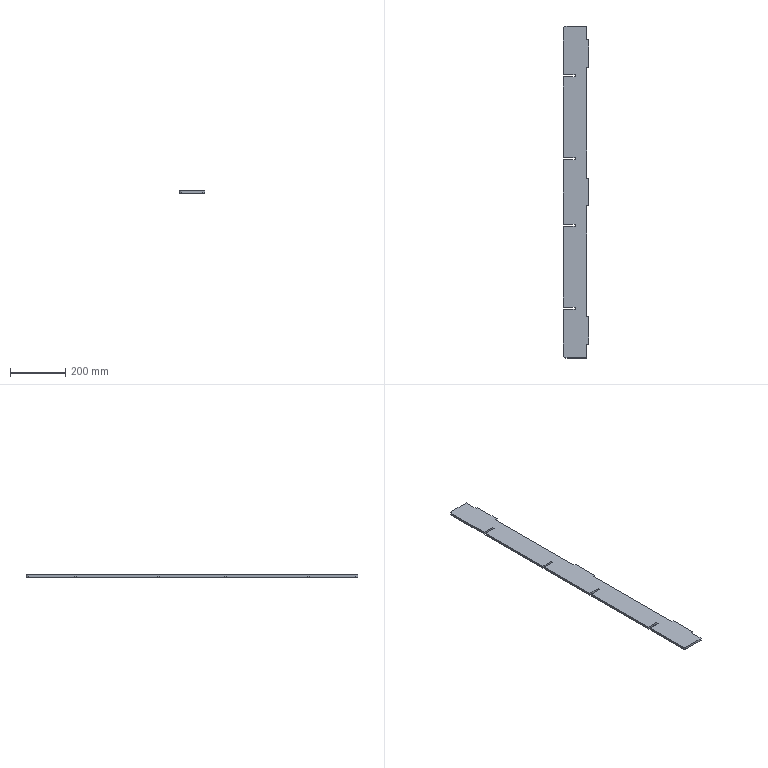Part | SolidWorks | features FlatPattern 1, SMBaseFlange 1, SheetMetal 1 | 1 solid | 36 faces | box 92.5 x 1200 x 8 mm | volume 822649 mm3 | plane 34 | cylinder 2 | commonest cylinder face diameters 20 x2
STEP:
#1=CARTESIAN_POINT('',(982.506,-540.938,0.));
#2=VERTEX_POINT('',#1);
#3=CARTESIAN_POINT('',(982.506,-490.938,0.));
#4=VERTEX_POINT('',#3);
#5=CARTESIAN_POINT('',(982.506,-490.938,0.));
#6=DIRECTION('',(0.,1.,0.));
#7=VECTOR('',#6,1000.);
#8=LINE('',#5,#7);
#9=EDGE_CURVE('',#2,#4,#8,.T.);
#10=ORIENTED_EDGE('',*,*,#9,.F.);
#11=CARTESIAN_POINT('',(982.506,-540.938,-8.));
#12=VERTEX_POINT('',#11);
#13=CARTESIAN_POINT('',(982.506,-540.938,-8.));
#14=DIRECTION('',(0.,0.,1.));
#15=VECTOR('',#14,1000.);
#16=LINE('',#13,#15);
#17=EDGE_CURVE('',#12,#2,#16,.T.);
#18=ORIENTED_EDGE('',*,*,#17,.F.);
#19=CARTESIAN_POINT('',(982.506,-490.938,-8.));
#20=VERTEX_POINT('',#19);
#21=CARTESIAN_POINT('',(982.506,-490.938,-8.));
#22=DIRECTION('',(0.,1.,0.));
#23=VECTOR('',#22,1000.);
#24=LINE('',#21,#23);
#25=EDGE_CURVE('',#12,#20,#24,.T.);
#26=ORIENTED_EDGE('',*,*,#25,.T.);
#27=CARTESIAN_POINT('',(982.506,-490.938,-8.));
#28=DIRECTION('',(0.,0.,1.));
#29=VECTOR('',#28,1000.);
#30=LINE('',#27,#29);
#31=EDGE_CURVE('',#20,#4,#30,.T.);
#32=ORIENTED_EDGE('',*,*,#31,.T.);
#33=EDGE_LOOP('',(#10,#18,#26,#32));
#34=FACE_OUTER_BOUND('',#33,.T.);
#35=CARTESIAN_POINT('',(982.506,-490.938,-8.));
#36=DIRECTION('',(1.,0.,0.));
#37=DIRECTION('',(0.,1.,0.));
#38=AXIS2_PLACEMENT_3D('',#35,#36,#37);
#39=PLANE('',#38);
#40=ADVANCED_FACE('',(#34),#39,.T.);
#41=CARTESIAN_POINT('',(907.506,-540.938,0.));
#42=VERTEX_POINT('',#41);
#43=CARTESIAN_POINT('',(982.506,-540.938,0.));
#44=DIRECTION('',(1.,0.,0.));
#45=VECTOR('',#44,1000.);
#46=LINE('',#43,#45);
#47=EDGE_CURVE('',#42,#2,#46,.T.);
#48=ORIENTED_EDGE('',*,*,#47,.F.);
#49=CARTESIAN_POINT('',(907.506,-540.938,-8.));
#50=VERTEX_POINT('',#49);
#51=CARTESIAN_POINT('',(907.506,-540.938,-8.));
#52=DIRECTION('',(0.,0.,1.));
#53=VECTOR('',#52,1000.);
#54=LINE('',#51,#53);
#55=EDGE_CURVE('',#50,#42,#54,.T.);
#56=ORIENTED_EDGE('',*,*,#55,.F.);
#57=CARTESIAN_POINT('',(982.506,-540.938,-8.));
#58=DIRECTION('',(1.,0.,0.));
#59=VECTOR('',#58,1000.);
#60=LINE('',#57,#59);
#61=EDGE_CURVE('',#50,#12,#60,.T.);
#62=ORIENTED_EDGE('',*,*,#61,.T.);
#63=ORIENTED_EDGE('',*,*,#17,.T.);
#64=EDGE_LOOP('',(#48,#56,#62,#63));
#65=FACE_OUTER_BOUND('',#64,.T.);
#66=CARTESIAN_POINT('',(982.506,-540.938,-8.));
#67=DIRECTION('',(0.,-1.,0.));
#68=DIRECTION('',(0.,0.,-1.));
#69=AXIS2_PLACEMENT_3D('',#66,#67,#68);
#70=PLANE('',#69);
#71=ADVANCED_FACE('',(#65),#70,.T.);
#72=CARTESIAN_POINT('',(897.506,-530.938,0.));
#73=VERTEX_POINT('',#72);
#74=CARTESIAN_POINT('',(907.506,-530.938,0.));
#75=DIRECTION('',(0.,0.,1.));
#76=DIRECTION('',(-1.,0.,0.));
#77=AXIS2_PLACEMENT_3D('',#74,#75,#76);
#78=CIRCLE('',#77,10.);
#79=EDGE_CURVE('',#73,#42,#78,.T.);
#80=ORIENTED_EDGE('',*,*,#79,.F.);
#81=CARTESIAN_POINT('',(897.506,-530.938,-8.));
#82=VERTEX_POINT('',#81);
#83=CARTESIAN_POINT('',(897.506,-530.938,-8.));
#84=DIRECTION('',(0.,0.,1.));
#85=VECTOR('',#84,1000.);
#86=LINE('',#83,#85);
#87=EDGE_CURVE('',#82,#73,#86,.T.);
#88=ORIENTED_EDGE('',*,*,#87,.F.);
#89=CARTESIAN_POINT('',(907.506,-530.938,-8.));
#90=DIRECTION('',(0.,0.,1.));
#91=DIRECTION('',(-1.,0.,0.));
#92=AXIS2_PLACEMENT_3D('',#89,#90,#91);
#93=CIRCLE('',#92,10.);
#94=EDGE_CURVE('',#82,#50,#93,.T.);
#95=ORIENTED_EDGE('',*,*,#94,.T.);
#96=ORIENTED_EDGE('',*,*,#55,.T.);
#97=EDGE_LOOP('',(#80,#88,#95,#96));
#98=FACE_OUTER_BOUND('',#97,.T.);
#99=CARTESIAN_POINT('',(907.506,-530.938,-8.));
#100=DIRECTION('',(0.,0.,1.));
#101=DIRECTION('',(1.,0.,0.));
#102=AXIS2_PLACEMENT_3D('',#99,#100,#101);
#103=CYLINDRICAL_SURFACE('',#102,10.);
#104=ADVANCED_FACE('',(#98),#103,.T.);
#105=CARTESIAN_POINT('',(897.506,-364.938,0.));
#106=VERTEX_POINT('',#105);
#107=CARTESIAN_POINT('',(897.506,-530.938,0.));
#108=DIRECTION('',(0.,-1.,0.));
#109=VECTOR('',#108,1000.);
#110=LINE('',#107,#109);
#111=EDGE_CURVE('',#106,#73,#110,.T.);
#112=ORIENTED_EDGE('',*,*,#111,.F.);
#113=CARTESIAN_POINT('',(897.506,-364.938,-8.));
#114=VERTEX_POINT('',#113);
#115=CARTESIAN_POINT('',(897.506,-364.938,-8.));
#116=DIRECTION('',(0.,0.,1.));
#117=VECTOR('',#116,1000.);
#118=LINE('',#115,#117);
#119=EDGE_CURVE('',#114,#106,#118,.T.);
#120=ORIENTED_EDGE('',*,*,#119,.F.);
#121=CARTESIAN_POINT('',(897.506,-530.938,-8.));
#122=DIRECTION('',(0.,-1.,0.));
#123=VECTOR('',#122,1000.);
#124=LINE('',#121,#123);
#125=EDGE_CURVE('',#114,#82,#124,.T.);
#126=ORIENTED_EDGE('',*,*,#125,.T.);
#127=ORIENTED_EDGE('',*,*,#87,.T.);
#128=EDGE_LOOP('',(#112,#120,#126,#127));
#129=FACE_OUTER_BOUND('',#128,.T.);
#130=CARTESIAN_POINT('',(897.506,-530.938,-8.));
#131=DIRECTION('',(-1.,0.,0.));
#132=DIRECTION('',(0.,0.,1.));
#133=AXIS2_PLACEMENT_3D('',#130,#131,#132);
#134=PLANE('',#133);
#135=ADVANCED_FACE('',(#129),#134,.T.);
#136=CARTESIAN_POINT('',(940.506,-364.938,0.));
#137=VERTEX_POINT('',#136);
#138=CARTESIAN_POINT('',(940.506,-364.938,0.));
#139=DIRECTION('',(-1.,0.,0.));
#140=VECTOR('',#139,1000.);
#141=LINE('',#138,#140);
#142=EDGE_CURVE('',#137,#106,#141,.T.);
#143=ORIENTED_EDGE('',*,*,#142,.F.);
#144=CARTESIAN_POINT('',(940.506,-364.938,-8.));
#145=VERTEX_POINT('',#144);
#146=CARTESIAN_POINT('',(940.506,-364.938,-8.));
#147=DIRECTION('',(0.,0.,1.));
#148=VECTOR('',#147,1000.);
#149=LINE('',#146,#148);
#150=EDGE_CURVE('',#145,#137,#149,.T.);
#151=ORIENTED_EDGE('',*,*,#150,.F.);
#152=CARTESIAN_POINT('',(940.506,-364.938,-8.));
#153=DIRECTION('',(-1.,0.,0.));
#154=VECTOR('',#153,1000.);
#155=LINE('',#152,#154);
#156=EDGE_CURVE('',#145,#114,#155,.T.);
#157=ORIENTED_EDGE('',*,*,#156,.T.);
#158=ORIENTED_EDGE('',*,*,#119,.T.);
#159=EDGE_LOOP('',(#143,#151,#157,#158));
#160=FACE_OUTER_BOUND('',#159,.T.);
#161=CARTESIAN_POINT('',(940.506,-364.938,-8.));
#162=DIRECTION('',(0.,1.,0.));
#163=DIRECTION('',(0.,0.,1.));
#164=AXIS2_PLACEMENT_3D('',#161,#162,#163);
#165=PLANE('',#164);
#166=ADVANCED_FACE('',(#160),#165,.T.);
#167=CARTESIAN_POINT('',(940.506,-356.938,0.));
#168=VERTEX_POINT('',#167);
#169=CARTESIAN_POINT('',(940.506,-356.938,0.));
#170=DIRECTION('',(0.,-1.,0.));
#171=VECTOR('',#170,1000.);
#172=LINE('',#169,#171);
#173=EDGE_CURVE('',#168,#137,#172,.T.);
#174=ORIENTED_EDGE('',*,*,#173,.F.);
#175=CARTESIAN_POINT('',(940.506,-356.938,-8.));
#176=VERTEX_POINT('',#175);
#177=CARTESIAN_POINT('',(940.506,-356.938,-8.));
#178=DIRECTION('',(0.,0.,1.));
#179=VECTOR('',#178,1000.);
#180=LINE('',#177,#179);
#181=EDGE_CURVE('',#176,#168,#180,.T.);
#182=ORIENTED_EDGE('',*,*,#181,.F.);
#183=CARTESIAN_POINT('',(940.506,-356.938,-8.));
#184=DIRECTION('',(0.,-1.,0.));
#185=VECTOR('',#184,1000.);
#186=LINE('',#183,#185);
#187=EDGE_CURVE('',#176,#145,#186,.T.);
#188=ORIENTED_EDGE('',*,*,#187,.T.);
#189=ORIENTED_EDGE('',*,*,#150,.T.);
#190=EDGE_LOOP('',(#174,#182,#188,#189));
#191=FACE_OUTER_BOUND('',#190,.T.);
#192=CARTESIAN_POINT('',(940.506,-356.938,-8.));
#193=DIRECTION('',(-1.,0.,0.));
#194=DIRECTION('',(0.,0.,1.));
#195=AXIS2_PLACEMENT_3D('',#192,#193,#194);
#196=PLANE('',#195);
#197=ADVANCED_FACE('',(#191),#196,.T.);
#198=CARTESIAN_POINT('',(897.506,-356.938,0.));
#199=VERTEX_POINT('',#198);
#200=CARTESIAN_POINT('',(897.506,-356.938,0.));
#201=DIRECTION('',(1.,0.,0.));
#202=VECTOR('',#201,1000.);
#203=LINE('',#200,#202);
#204=EDGE_CURVE('',#199,#168,#203,.T.);
#205=ORIENTED_EDGE('',*,*,#204,.F.);
#206=CARTESIAN_POINT('',(897.506,-356.938,-8.));
#207=VERTEX_POINT('',#206);
#208=CARTESIAN_POINT('',(897.506,-356.938,-8.));
#209=DIRECTION('',(0.,0.,1.));
#210=VECTOR('',#209,1000.);
#211=LINE('',#208,#210);
#212=EDGE_CURVE('',#207,#199,#211,.T.);
#213=ORIENTED_EDGE('',*,*,#212,.F.);
#214=CARTESIAN_POINT('',(897.506,-356.938,-8.));
#215=DIRECTION('',(1.,0.,0.));
#216=VECTOR('',#215,1000.);
#217=LINE('',#214,#216);
#218=EDGE_CURVE('',#207,#176,#217,.T.);
#219=ORIENTED_EDGE('',*,*,#218,.T.);
#220=ORIENTED_EDGE('',*,*,#181,.T.);
#221=EDGE_LOOP('',(#205,#213,#219,#220));
#222=FACE_OUTER_BOUND('',#221,.T.);
#223=CARTESIAN_POINT('',(897.506,-356.938,-8.));
#224=DIRECTION('',(0.,-1.,0.));
#225=DIRECTION('',(0.,0.,-1.));
#226=AXIS2_PLACEMENT_3D('',#223,#224,#225);
#227=PLANE('',#226);
#228=ADVANCED_FACE('',(#222),#227,.T.);
#229=CARTESIAN_POINT('',(897.506,-64.938,0.));
#230=VERTEX_POINT('',#229);
#231=CARTESIAN_POINT('',(897.506,-356.938,0.));
#232=DIRECTION('',(0.,-1.,0.));
#233=VECTOR('',#232,1000.);
#234=LINE('',#231,#233);
#235=EDGE_CURVE('',#230,#199,#234,.T.);
#236=ORIENTED_EDGE('',*,*,#235,.F.);
#237=CARTESIAN_POINT('',(897.506,-64.938,-8.));
#238=VERTEX_POINT('',#237);
#239=CARTESIAN_POINT('',(897.506,-64.938,-8.));
#240=DIRECTION('',(0.,0.,1.));
#241=VECTOR('',#240,1000.);
#242=LINE('',#239,#241);
#243=EDGE_CURVE('',#238,#230,#242,.T.);
#244=ORIENTED_EDGE('',*,*,#243,.F.);
#245=CARTESIAN_POINT('',(897.506,-356.938,-8.));
#246=DIRECTION('',(0.,-1.,0.));
#247=VECTOR('',#246,1000.);
#248=LINE('',#245,#247);
#249=EDGE_CURVE('',#238,#207,#248,.T.);
#250=ORIENTED_EDGE('',*,*,#249,.T.);
#251=ORIENTED_EDGE('',*,*,#212,.T.);
#252=EDGE_LOOP('',(#236,#244,#250,#251));
#253=FACE_OUTER_BOUND('',#252,.T.);
#254=CARTESIAN_POINT('',(897.506,-356.938,-8.));
#255=DIRECTION('',(-1.,0.,0.));
#256=DIRECTION('',(0.,0.,1.));
#257=AXIS2_PLACEMENT_3D('',#254,#255,#256);
#258=PLANE('',#257);
#259=ADVANCED_FACE('',(#253),#258,.T.);
#260=CARTESIAN_POINT('',(940.506,-64.938,0.));
#261=VERTEX_POINT('',#260);
#262=CARTESIAN_POINT('',(940.506,-64.938,0.));
#263=DIRECTION('',(-1.,0.,0.));
#264=VECTOR('',#263,1000.);
#265=LINE('',#262,#264);
#266=EDGE_CURVE('',#261,#230,#265,.T.);
#267=ORIENTED_EDGE('',*,*,#266,.F.);
#268=CARTESIAN_POINT('',(940.506,-64.938,-8.));
#269=VERTEX_POINT('',#268);
#270=CARTESIAN_POINT('',(940.506,-64.938,-8.));
#271=DIRECTION('',(0.,0.,1.));
#272=VECTOR('',#271,1000.);
#273=LINE('',#270,#272);
#274=EDGE_CURVE('',#269,#261,#273,.T.);
#275=ORIENTED_EDGE('',*,*,#274,.F.);
#276=CARTESIAN_POINT('',(940.506,-64.938,-8.));
#277=DIRECTION('',(-1.,0.,0.));
#278=VECTOR('',#277,1000.);
#279=LINE('',#276,#278);
#280=EDGE_CURVE('',#269,#238,#279,.T.);
#281=ORIENTED_EDGE('',*,*,#280,.T.);
#282=ORIENTED_EDGE('',*,*,#243,.T.);
#283=EDGE_LOOP('',(#267,#275,#281,#282));
#284=FACE_OUTER_BOUND('',#283,.T.);
#285=CARTESIAN_POINT('',(940.506,-64.938,-8.));
#286=DIRECTION('',(0.,1.,0.));
#287=DIRECTION('',(0.,0.,1.));
#288=AXIS2_PLACEMENT_3D('',#285,#286,#287);
#289=PLANE('',#288);
#290=ADVANCED_FACE('',(#284),#289,.T.);
#291=CARTESIAN_POINT('',(940.506,-56.938,0.));
#292=VERTEX_POINT('',#291);
#293=CARTESIAN_POINT('',(940.506,-56.938,0.));
#294=DIRECTION('',(0.,-1.,0.));
#295=VECTOR('',#294,1000.);
#296=LINE('',#293,#295);
#297=EDGE_CURVE('',#292,#261,#296,.T.);
#298=ORIENTED_EDGE('',*,*,#297,.F.);
#299=CARTESIAN_POINT('',(940.506,-56.938,-8.));
#300=VERTEX_POINT('',#299);
#301=CARTESIAN_POINT('',(940.506,-56.938,-8.));
#302=DIRECTION('',(0.,0.,1.));
#303=VECTOR('',#302,1000.);
#304=LINE('',#301,#303);
#305=EDGE_CURVE('',#300,#292,#304,.T.);
#306=ORIENTED_EDGE('',*,*,#305,.F.);
#307=CARTESIAN_POINT('',(940.506,-56.938,-8.));
#308=DIRECTION('',(0.,-1.,0.));
#309=VECTOR('',#308,1000.);
#310=LINE('',#307,#309);
#311=EDGE_CURVE('',#300,#269,#310,.T.);
#312=ORIENTED_EDGE('',*,*,#311,.T.);
#313=ORIENTED_EDGE('',*,*,#274,.T.);
#314=EDGE_LOOP('',(#298,#306,#312,#313));
#315=FACE_OUTER_BOUND('',#314,.T.);
#316=CARTESIAN_POINT('',(940.506,-56.938,-8.));
#317=DIRECTION('',(-1.,0.,0.));
#318=DIRECTION('',(0.,0.,1.));
#319=AXIS2_PLACEMENT_3D('',#316,#317,#318);
#320=PLANE('',#319);
#321=ADVANCED_FACE('',(#315),#320,.T.);
#322=CARTESIAN_POINT('',(897.506,-56.938,0.));
#323=VERTEX_POINT('',#322);
#324=CARTESIAN_POINT('',(897.506,-56.938,0.));
#325=DIRECTION('',(1.,0.,0.));
#326=VECTOR('',#325,1000.);
#327=LINE('',#324,#326);
#328=EDGE_CURVE('',#323,#292,#327,.T.);
#329=ORIENTED_EDGE('',*,*,#328,.F.);
#330=CARTESIAN_POINT('',(897.506,-56.938,-8.));
#331=VERTEX_POINT('',#330);
#332=CARTESIAN_POINT('',(897.506,-56.938,-8.));
#333=DIRECTION('',(0.,0.,1.));
#334=VECTOR('',#333,1000.);
#335=LINE('',#332,#334);
#336=EDGE_CURVE('',#331,#323,#335,.T.);
#337=ORIENTED_EDGE('',*,*,#336,.F.);
#338=CARTESIAN_POINT('',(897.506,-56.938,-8.));
#339=DIRECTION('',(1.,0.,0.));
#340=VECTOR('',#339,1000.);
#341=LINE('',#338,#340);
#342=EDGE_CURVE('',#331,#300,#341,.T.);
#343=ORIENTED_EDGE('',*,*,#342,.T.);
#344=ORIENTED_EDGE('',*,*,#305,.T.);
#345=EDGE_LOOP('',(#329,#337,#343,#344));
#346=FACE_OUTER_BOUND('',#345,.T.);
#347=CARTESIAN_POINT('',(897.506,-56.938,-8.));
#348=DIRECTION('',(0.,-1.,0.));
#349=DIRECTION('',(0.,0.,-1.));
#350=AXIS2_PLACEMENT_3D('',#347,#348,#349);
#351=PLANE('',#350);
#352=ADVANCED_FACE('',(#346),#351,.T.);
#353=CARTESIAN_POINT('',(897.506,175.062,0.));
#354=VERTEX_POINT('',#353);
#355=CARTESIAN_POINT('',(897.506,-56.938,0.));
#356=DIRECTION('',(0.,-1.,0.));
#357=VECTOR('',#356,1000.);
#358=LINE('',#355,#357);
#359=EDGE_CURVE('',#354,#323,#358,.T.);
#360=ORIENTED_EDGE('',*,*,#359,.F.);
#361=CARTESIAN_POINT('',(897.506,175.062,-8.));
#362=VERTEX_POINT('',#361);
#363=CARTESIAN_POINT('',(897.506,175.062,-8.));
#364=DIRECTION('',(0.,0.,1.));
#365=VECTOR('',#364,1000.);
#366=LINE('',#363,#365);
#367=EDGE_CURVE('',#362,#354,#366,.T.);
#368=ORIENTED_EDGE('',*,*,#367,.F.);
#369=CARTESIAN_POINT('',(897.506,-56.938,-8.));
#370=DIRECTION('',(0.,-1.,0.));
#371=VECTOR('',#370,1000.);
#372=LINE('',#369,#371);
#373=EDGE_CURVE('',#362,#331,#372,.T.);
#374=ORIENTED_EDGE('',*,*,#373,.T.);
#375=ORIENTED_EDGE('',*,*,#336,.T.);
#376=EDGE_LOOP('',(#360,#368,#374,#375));
#377=FACE_OUTER_BOUND('',#376,.T.);
#378=CARTESIAN_POINT('',(897.506,-56.938,-8.));
#379=DIRECTION('',(-1.,0.,0.));
#380=DIRECTION('',(0.,0.,1.));
#381=AXIS2_PLACEMENT_3D('',#378,#379,#380);
#382=PLANE('',#381);
#383=ADVANCED_FACE('',(#377),#382,.T.);
#384=CARTESIAN_POINT('',(940.506,175.062,0.));
#385=VERTEX_POINT('',#384);
#386=CARTESIAN_POINT('',(940.506,175.062,0.));
#387=DIRECTION('',(-1.,0.,0.));
#388=VECTOR('',#387,1000.);
#389=LINE('',#386,#388);
#390=EDGE_CURVE('',#385,#354,#389,.T.);
#391=ORIENTED_EDGE('',*,*,#390,.F.);
#392=CARTESIAN_POINT('',(940.506,175.062,-8.));
#393=VERTEX_POINT('',#392);
#394=CARTESIAN_POINT('',(940.506,175.062,-8.));
#395=DIRECTION('',(0.,0.,1.));
#396=VECTOR('',#395,1000.);
#397=LINE('',#394,#396);
#398=EDGE_CURVE('',#393,#385,#397,.T.);
#399=ORIENTED_EDGE('',*,*,#398,.F.);
#400=CARTESIAN_POINT('',(940.506,175.062,-8.));
#401=DIRECTION('',(-1.,0.,0.));
#402=VECTOR('',#401,1000.);
#403=LINE('',#400,#402);
#404=EDGE_CURVE('',#393,#362,#403,.T.);
#405=ORIENTED_EDGE('',*,*,#404,.T.);
#406=ORIENTED_EDGE('',*,*,#367,.T.);
#407=EDGE_LOOP('',(#391,#399,#405,#406));
#408=FACE_OUTER_BOUND('',#407,.T.);
#409=CARTESIAN_POINT('',(940.506,175.062,-8.));
#410=DIRECTION('',(0.,1.,0.));
#411=DIRECTION('',(0.,0.,1.));
#412=AXIS2_PLACEMENT_3D('',#409,#410,#411);
#413=PLANE('',#412);
#414=ADVANCED_FACE('',(#408),#413,.T.);
#415=CARTESIAN_POINT('',(940.506,183.062,0.));
#416=VERTEX_POINT('',#415);
#417=CARTESIAN_POINT('',(940.506,183.062,0.));
#418=DIRECTION('',(0.,-1.,0.));
#419=VECTOR('',#418,1000.);
#420=LINE('',#417,#419);
#421=EDGE_CURVE('',#416,#385,#420,.T.);
#422=ORIENTED_EDGE('',*,*,#421,.F.);
#423=CARTESIAN_POINT('',(940.506,183.062,-8.));
#424=VERTEX_POINT('',#423);
#425=CARTESIAN_POINT('',(940.506,183.062,-8.));
#426=DIRECTION('',(0.,0.,1.));
#427=VECTOR('',#426,1000.);
#428=LINE('',#425,#427);
#429=EDGE_CURVE('',#424,#416,#428,.T.);
#430=ORIENTED_EDGE('',*,*,#429,.F.);
#431=CARTESIAN_POINT('',(940.506,183.062,-8.));
#432=DIRECTION('',(0.,-1.,0.));
#433=VECTOR('',#432,1000.);
#434=LINE('',#431,#433);
#435=EDGE_CURVE('',#424,#393,#434,.T.);
#436=ORIENTED_EDGE('',*,*,#435,.T.);
#437=ORIENTED_EDGE('',*,*,#398,.T.);
#438=EDGE_LOOP('',(#422,#430,#436,#437));
#439=FACE_OUTER_BOUND('',#438,.T.);
#440=CARTESIAN_POINT('',(940.506,183.062,-8.));
#441=DIRECTION('',(-1.,0.,0.));
#442=DIRECTION('',(0.,0.,1.));
#443=AXIS2_PLACEMENT_3D('',#440,#441,#442);
#444=PLANE('',#443);
#445=ADVANCED_FACE('',(#439),#444,.T.);
#446=CARTESIAN_POINT('',(897.506,183.062,0.));
#447=VERTEX_POINT('',#446);
#448=CARTESIAN_POINT('',(897.506,183.062,0.));
#449=DIRECTION('',(1.,0.,0.));
#450=VECTOR('',#449,1000.);
#451=LINE('',#448,#450);
#452=EDGE_CURVE('',#447,#416,#451,.T.);
#453=ORIENTED_EDGE('',*,*,#452,.F.);
#454=CARTESIAN_POINT('',(897.506,183.062,-8.));
#455=VERTEX_POINT('',#454);
#456=CARTESIAN_POINT('',(897.506,183.062,-8.));
#457=DIRECTION('',(0.,0.,1.));
#458=VECTOR('',#457,1000.);
#459=LINE('',#456,#458);
#460=EDGE_CURVE('',#455,#447,#459,.T.);
#461=ORIENTED_EDGE('',*,*,#460,.F.);
#462=CARTESIAN_POINT('',(897.506,183.062,-8.));
#463=DIRECTION('',(1.,0.,0.));
#464=VECTOR('',#463,1000.);
#465=LINE('',#462,#464);
#466=EDGE_CURVE('',#455,#424,#465,.T.);
#467=ORIENTED_EDGE('',*,*,#466,.T.);
#468=ORIENTED_EDGE('',*,*,#429,.T.);
#469=EDGE_LOOP('',(#453,#461,#467,#468));
#470=FACE_OUTER_BOUND('',#469,.T.);
#471=CARTESIAN_POINT('',(897.506,183.062,-8.));
#472=DIRECTION('',(0.,-1.,0.));
#473=DIRECTION('',(1.,0.,0.));
#474=AXIS2_PLACEMENT_3D('',#471,#472,#473);
#475=PLANE('',#474);
#476=ADVANCED_FACE('',(#470),#475,.T.);
#477=CARTESIAN_POINT('',(897.506,475.062,0.));
#478=VERTEX_POINT('',#477);
#479=CARTESIAN_POINT('',(897.506,183.062,0.));
#480=DIRECTION('',(0.,-1.,0.));
#481=VECTOR('',#480,1000.);
#482=LINE('',#479,#481);
#483=EDGE_CURVE('',#478,#447,#482,.T.);
#484=ORIENTED_EDGE('',*,*,#483,.F.);
#485=CARTESIAN_POINT('',(897.506,475.062,-8.));
#486=VERTEX_POINT('',#485);
#487=CARTESIAN_POINT('',(897.506,475.062,-8.));
#488=DIRECTION('',(0.,0.,1.));
#489=VECTOR('',#488,1000.);
#490=LINE('',#487,#489);
#491=EDGE_CURVE('',#486,#478,#490,.T.);
#492=ORIENTED_EDGE('',*,*,#491,.F.);
#493=CARTESIAN_POINT('',(897.506,183.062,-8.));
#494=DIRECTION('',(0.,-1.,0.));
#495=VECTOR('',#494,1000.);
#496=LINE('',#493,#495);
#497=EDGE_CURVE('',#486,#455,#496,.T.);
#498=ORIENTED_EDGE('',*,*,#497,.T.);
#499=ORIENTED_EDGE('',*,*,#460,.T.);
#500=EDGE_LOOP('',(#484,#492,#498,#499));
#501=FACE_OUTER_BOUND('',#500,.T.);
#502=CARTESIAN_POINT('',(897.506,183.062,-8.));
#503=DIRECTION('',(-1.,0.,0.));
#504=DIRECTION('',(0.,0.,1.));
#505=AXIS2_PLACEMENT_3D('',#502,#503,#504);
#506=PLANE('',#505);
#507=ADVANCED_FACE('',(#501),#506,.T.);
#508=CARTESIAN_POINT('',(940.506,475.062,0.));
#509=VERTEX_POINT('',#508);
#510=CARTESIAN_POINT('',(940.506,475.062,0.));
#511=DIRECTION('',(-1.,0.,0.));
#512=VECTOR('',#511,1000.);
#513=LINE('',#510,#512);
#514=EDGE_CURVE('',#509,#478,#513,.T.);
#515=ORIENTED_EDGE('',*,*,#514,.F.);
#516=CARTESIAN_POINT('',(940.506,475.062,-8.));
#517=VERTEX_POINT('',#516);
#518=CARTESIAN_POINT('',(940.506,475.062,-8.));
#519=DIRECTION('',(0.,0.,1.));
#520=VECTOR('',#519,1000.);
#521=LINE('',#518,#520);
#522=EDGE_CURVE('',#517,#509,#521,.T.);
#523=ORIENTED_EDGE('',*,*,#522,.F.);
#524=CARTESIAN_POINT('',(940.506,475.062,-8.));
#525=DIRECTION('',(-1.,0.,0.));
#526=VECTOR('',#525,1000.);
#527=LINE('',#524,#526);
#528=EDGE_CURVE('',#517,#486,#527,.T.);
#529=ORIENTED_EDGE('',*,*,#528,.T.);
#530=ORIENTED_EDGE('',*,*,#491,.T.);
#531=EDGE_LOOP('',(#515,#523,#529,#530));
#532=FACE_OUTER_BOUND('',#531,.T.);
#533=CARTESIAN_POINT('',(940.506,475.062,-8.));
#534=DIRECTION('',(0.,1.,0.));
#535=DIRECTION('',(-1.,0.,0.));
#536=AXIS2_PLACEMENT_3D('',#533,#534,#535);
#537=PLANE('',#536);
#538=ADVANCED_FACE('',(#532),#537,.T.);
#539=CARTESIAN_POINT('',(940.506,483.062,0.));
#540=VERTEX_POINT('',#539);
#541=CARTESIAN_POINT('',(940.506,483.062,0.));
#542=DIRECTION('',(0.,-1.,0.));
#543=VECTOR('',#542,1000.);
#544=LINE('',#541,#543);
#545=EDGE_CURVE('',#540,#509,#544,.T.);
#546=ORIENTED_EDGE('',*,*,#545,.F.);
#547=CARTESIAN_POINT('',(940.506,483.062,-8.));
#548=VERTEX_POINT('',#547);
#549=CARTESIAN_POINT('',(940.506,483.062,-8.));
#550=DIRECTION('',(0.,0.,1.));
#551=VECTOR('',#550,1000.);
#552=LINE('',#549,#551);
#553=EDGE_CURVE('',#548,#540,#552,.T.);
#554=ORIENTED_EDGE('',*,*,#553,.F.);
#555=CARTESIAN_POINT('',(940.506,483.062,-8.));
#556=DIRECTION('',(0.,-1.,0.));
#557=VECTOR('',#556,1000.);
#558=LINE('',#555,#557);
#559=EDGE_CURVE('',#548,#517,#558,.T.);
#560=ORIENTED_EDGE('',*,*,#559,.T.);
#561=ORIENTED_EDGE('',*,*,#522,.T.);
#562=EDGE_LOOP('',(#546,#554,#560,#561));
#563=FACE_OUTER_BOUND('',#562,.T.);
#564=CARTESIAN_POINT('',(940.506,483.062,-8.));
#565=DIRECTION('',(-1.,0.,0.));
#566=DIRECTION('',(0.,0.,1.));
#567=AXIS2_PLACEMENT_3D('',#564,#565,#566);
#568=PLANE('',#567);
#569=ADVANCED_FACE('',(#563),#568,.T.);
#570=CARTESIAN_POINT('',(897.506,483.062,0.));
#571=VERTEX_POINT('',#570);
#572=CARTESIAN_POINT('',(897.506,483.062,0.));
#573=DIRECTION('',(1.,0.,0.));
#574=VECTOR('',#573,1000.);
#575=LINE('',#572,#574);
#576=EDGE_CURVE('',#571,#540,#575,.T.);
#577=ORIENTED_EDGE('',*,*,#576,.F.);
#578=CARTESIAN_POINT('',(897.506,483.062,-8.));
#579=VERTEX_POINT('',#578);
#580=CARTESIAN_POINT('',(897.506,483.062,-8.));
#581=DIRECTION('',(0.,0.,1.));
#582=VECTOR('',#581,1000.);
#583=LINE('',#580,#582);
#584=EDGE_CURVE('',#579,#571,#583,.T.);
#585=ORIENTED_EDGE('',*,*,#584,.F.);
#586=CARTESIAN_POINT('',(897.506,483.062,-8.));
#587=DIRECTION('',(1.,0.,0.));
#588=VECTOR('',#587,1000.);
#589=LINE('',#586,#588);
#590=EDGE_CURVE('',#579,#548,#589,.T.);
#591=ORIENTED_EDGE('',*,*,#590,.T.);
#592=ORIENTED_EDGE('',*,*,#553,.T.);
#593=EDGE_LOOP('',(#577,#585,#591,#592));
#594=FACE_OUTER_BOUND('',#593,.T.);
#595=CARTESIAN_POINT('',(897.506,483.062,-8.));
#596=DIRECTION('',(0.,-1.,0.));
#597=DIRECTION('',(1.,0.,0.));
#598=AXIS2_PLACEMENT_3D('',#595,#596,#597);
#599=PLANE('',#598);
#600=ADVANCED_FACE('',(#594),#599,.T.);
#601=CARTESIAN_POINT('',(897.506,649.062,0.));
#602=VERTEX_POINT('',#601);
#603=CARTESIAN_POINT('',(897.506,483.062,0.));
#604=DIRECTION('',(0.,-1.,0.));
#605=VECTOR('',#604,1000.);
#606=LINE('',#603,#605);
#607=EDGE_CURVE('',#602,#571,#606,.T.);
#608=ORIENTED_EDGE('',*,*,#607,.F.);
#609=CARTESIAN_POINT('',(897.506,649.062,-8.));
#610=VERTEX_POINT('',#609);
#611=CARTESIAN_POINT('',(897.506,649.062,-8.));
#612=DIRECTION('',(0.,0.,1.));
#613=VECTOR('',#612,1000.);
#614=LINE('',#611,#613);
#615=EDGE_CURVE('',#610,#602,#614,.T.);
#616=ORIENTED_EDGE('',*,*,#615,.F.);
#617=CARTESIAN_POINT('',(897.506,483.062,-8.));
#618=DIRECTION('',(0.,-1.,0.));
#619=VECTOR('',#618,1000.);
#620=LINE('',#617,#619);
#621=EDGE_CURVE('',#610,#579,#620,.T.);
#622=ORIENTED_EDGE('',*,*,#621,.T.);
#623=ORIENTED_EDGE('',*,*,#584,.T.);
#624=EDGE_LOOP('',(#608,#616,#622,#623));
#625=FACE_OUTER_BOUND('',#624,.T.);
#626=CARTESIAN_POINT('',(897.506,483.062,-8.));
#627=DIRECTION('',(-1.,0.,0.));
#628=DIRECTION('',(0.,0.,1.));
#629=AXIS2_PLACEMENT_3D('',#626,#627,#628);
#630=PLANE('',#629);
#631=ADVANCED_FACE('',(#625),#630,.T.);
#632=CARTESIAN_POINT('',(907.506,659.062,0.));
#633=VERTEX_POINT('',#632);
#634=CARTESIAN_POINT('',(907.506,649.062,0.));
#635=DIRECTION('',(0.,0.,1.));
#636=DIRECTION('',(-1.,0.,0.));
#637=AXIS2_PLACEMENT_3D('',#634,#635,#636);
#638=CIRCLE('',#637,10.);
#639=EDGE_CURVE('',#633,#602,#638,.T.);
#640=ORIENTED_EDGE('',*,*,#639,.F.);
#641=CARTESIAN_POINT('',(907.506,659.062,-8.));
#642=VERTEX_POINT('',#641);
#643=CARTESIAN_POINT('',(907.506,659.062,-8.));
#644=DIRECTION('',(0.,0.,1.));
#645=VECTOR('',#644,1000.);
#646=LINE('',#643,#645);
#647=EDGE_CURVE('',#642,#633,#646,.T.);
#648=ORIENTED_EDGE('',*,*,#647,.F.);
#649=CARTESIAN_POINT('',(907.506,649.062,-8.));
#650=DIRECTION('',(0.,0.,1.));
#651=DIRECTION('',(-1.,0.,0.));
#652=AXIS2_PLACEMENT_3D('',#649,#650,#651);
#653=CIRCLE('',#652,10.);
#654=EDGE_CURVE('',#642,#610,#653,.T.);
#655=ORIENTED_EDGE('',*,*,#654,.T.);
#656=ORIENTED_EDGE('',*,*,#615,.T.);
#657=EDGE_LOOP('',(#640,#648,#655,#656));
#658=FACE_OUTER_BOUND('',#657,.T.);
#659=CARTESIAN_POINT('',(907.506,649.062,-8.));
#660=DIRECTION('',(0.,0.,1.));
#661=DIRECTION('',(1.,0.,0.));
#662=AXIS2_PLACEMENT_3D('',#659,#660,#661);
#663=CYLINDRICAL_SURFACE('',#662,10.);
#664=ADVANCED_FACE('',(#658),#663,.T.);
#665=CARTESIAN_POINT('',(982.506,659.062,0.));
#666=VERTEX_POINT('',#665);
#667=CARTESIAN_POINT('',(907.506,659.062,0.));
#668=DIRECTION('',(-1.,0.,0.));
#669=VECTOR('',#668,1000.);
#670=LINE('',#667,#669);
#671=EDGE_CURVE('',#666,#633,#670,.T.);
#672=ORIENTED_EDGE('',*,*,#671,.F.);
#673=CARTESIAN_POINT('',(982.506,659.062,-8.));
#674=VERTEX_POINT('',#673);
#675=CARTESIAN_POINT('',(982.506,659.062,-8.));
#676=DIRECTION('',(0.,0.,1.));
#677=VECTOR('',#676,1000.);
#678=LINE('',#675,#677);
#679=EDGE_CURVE('',#674,#666,#678,.T.);
#680=ORIENTED_EDGE('',*,*,#679,.F.);
#681=CARTESIAN_POINT('',(907.506,659.062,-8.));
#682=DIRECTION('',(-1.,0.,0.));
#683=VECTOR('',#682,1000.);
#684=LINE('',#681,#683);
#685=EDGE_CURVE('',#674,#642,#684,.T.);
#686=ORIENTED_EDGE('',*,*,#685,.T.);
#687=ORIENTED_EDGE('',*,*,#647,.T.);
#688=EDGE_LOOP('',(#672,#680,#686,#687));
#689=FACE_OUTER_BOUND('',#688,.T.);
#690=CARTESIAN_POINT('',(907.506,659.062,-8.));
#691=DIRECTION('',(0.,1.,0.));
#692=DIRECTION('',(0.,0.,1.));
#693=AXIS2_PLACEMENT_3D('',#690,#691,#692);
#694=PLANE('',#693);
#695=ADVANCED_FACE('',(#689),#694,.T.);
#696=CARTESIAN_POINT('',(982.506,609.062,0.));
#697=VERTEX_POINT('',#696);
#698=CARTESIAN_POINT('',(982.506,659.062,0.));
#699=DIRECTION('',(0.,1.,0.));
#700=VECTOR('',#699,1000.);
#701=LINE('',#698,#700);
#702=EDGE_CURVE('',#697,#666,#701,.T.);
#703=ORIENTED_EDGE('',*,*,#702,.F.);
#704=CARTESIAN_POINT('',(982.506,609.062,-8.));
#705=VERTEX_POINT('',#704);
#706=CARTESIAN_POINT('',(982.506,609.062,-8.));
#707=DIRECTION('',(0.,0.,1.));
#708=VECTOR('',#707,1000.);
#709=LINE('',#706,#708);
#710=EDGE_CURVE('',#705,#697,#709,.T.);
#711=ORIENTED_EDGE('',*,*,#710,.F.);
#712=CARTESIAN_POINT('',(982.506,659.062,-8.));
#713=DIRECTION('',(0.,1.,0.));
#714=VECTOR('',#713,1000.);
#715=LINE('',#712,#714);
#716=EDGE_CURVE('',#705,#674,#715,.T.);
#717=ORIENTED_EDGE('',*,*,#716,.T.);
#718=ORIENTED_EDGE('',*,*,#679,.T.);
#719=EDGE_LOOP('',(#703,#711,#717,#718));
#720=FACE_OUTER_BOUND('',#719,.T.);
#721=CARTESIAN_POINT('',(982.506,659.062,-8.));
#722=DIRECTION('',(1.,0.,0.));
#723=DIRECTION('',(0.,1.,0.));
#724=AXIS2_PLACEMENT_3D('',#721,#722,#723);
#725=PLANE('',#724);
#726=ADVANCED_FACE('',(#720),#725,.T.);
#727=CARTESIAN_POINT('',(990.006,609.062,0.));
#728=VERTEX_POINT('',#727);
#729=CARTESIAN_POINT('',(982.506,609.062,0.));
#730=DIRECTION('',(-1.,0.,0.));
#731=VECTOR('',#730,1000.);
#732=LINE('',#729,#731);
#733=EDGE_CURVE('',#728,#697,#732,.T.);
#734=ORIENTED_EDGE('',*,*,#733,.F.);
#735=CARTESIAN_POINT('',(990.006,609.062,-8.));
#736=VERTEX_POINT('',#735);
#737=CARTESIAN_POINT('',(990.006,609.062,-8.));
#738=DIRECTION('',(0.,0.,1.));
#739=VECTOR('',#738,1000.);
#740=LINE('',#737,#739);
#741=EDGE_CURVE('',#736,#728,#740,.T.);
#742=ORIENTED_EDGE('',*,*,#741,.F.);
#743=CARTESIAN_POINT('',(982.506,609.062,-8.));
#744=DIRECTION('',(-1.,0.,0.));
#745=VECTOR('',#744,1000.);
#746=LINE('',#743,#745);
#747=EDGE_CURVE('',#736,#705,#746,.T.);
#748=ORIENTED_EDGE('',*,*,#747,.T.);
#749=ORIENTED_EDGE('',*,*,#710,.T.);
#750=EDGE_LOOP('',(#734,#742,#748,#749));
#751=FACE_OUTER_BOUND('',#750,.T.);
#752=CARTESIAN_POINT('',(982.506,609.062,-8.));
#753=DIRECTION('',(0.,1.,0.));
#754=DIRECTION('',(0.,0.,1.));
#755=AXIS2_PLACEMENT_3D('',#752,#753,#754);
#756=PLANE('',#755);
#757=ADVANCED_FACE('',(#751),#756,.T.);
#758=CARTESIAN_POINT('',(990.006,509.062,0.));
#759=VERTEX_POINT('',#758);
#760=CARTESIAN_POINT('',(990.006,609.062,0.));
#761=DIRECTION('',(0.,1.,0.));
#762=VECTOR('',#761,1000.);
#763=LINE('',#760,#762);
#764=EDGE_CURVE('',#759,#728,#763,.T.);
#765=ORIENTED_EDGE('',*,*,#764,.F.);
#766=CARTESIAN_POINT('',(990.006,509.062,-8.));
#767=VERTEX_POINT('',#766);
#768=CARTESIAN_POINT('',(990.006,509.062,-8.));
#769=DIRECTION('',(0.,0.,1.));
#770=VECTOR('',#769,1000.);
#771=LINE('',#768,#770);
#772=EDGE_CURVE('',#767,#759,#771,.T.);
#773=ORIENTED_EDGE('',*,*,#772,.F.);
#774=CARTESIAN_POINT('',(990.006,609.062,-8.));
#775=DIRECTION('',(0.,1.,0.));
#776=VECTOR('',#775,1000.);
#777=LINE('',#774,#776);
#778=EDGE_CURVE('',#767,#736,#777,.T.);
#779=ORIENTED_EDGE('',*,*,#778,.T.);
#780=ORIENTED_EDGE('',*,*,#741,.T.);
#781=EDGE_LOOP('',(#765,#773,#779,#780));
#782=FACE_OUTER_BOUND('',#781,.T.);
#783=CARTESIAN_POINT('',(990.006,609.062,-8.));
#784=DIRECTION('',(1.,0.,0.));
#785=DIRECTION('',(0.,0.,-1.));
#786=AXIS2_PLACEMENT_3D('',#783,#784,#785);
#787=PLANE('',#786);
#788=ADVANCED_FACE('',(#782),#787,.T.);
#789=CARTESIAN_POINT('',(982.506,509.062,0.));
#790=VERTEX_POINT('',#789);
#791=CARTESIAN_POINT('',(990.006,509.062,0.));
#792=DIRECTION('',(1.,0.,0.));
#793=VECTOR('',#792,1000.);
#794=LINE('',#791,#793);
#795=EDGE_CURVE('',#790,#759,#794,.T.);
#796=ORIENTED_EDGE('',*,*,#795,.F.);
#797=CARTESIAN_POINT('',(982.506,509.062,-8.));
#798=VERTEX_POINT('',#797);
#799=CARTESIAN_POINT('',(982.506,509.062,-8.));
#800=DIRECTION('',(0.,0.,1.));
#801=VECTOR('',#800,1000.);
#802=LINE('',#799,#801);
#803=EDGE_CURVE('',#798,#790,#802,.T.);
#804=ORIENTED_EDGE('',*,*,#803,.F.);
#805=CARTESIAN_POINT('',(990.006,509.062,-8.));
#806=DIRECTION('',(1.,0.,0.));
#807=VECTOR('',#806,1000.);
#808=LINE('',#805,#807);
#809=EDGE_CURVE('',#798,#767,#808,.T.);
#810=ORIENTED_EDGE('',*,*,#809,.T.);
#811=ORIENTED_EDGE('',*,*,#772,.T.);
#812=EDGE_LOOP('',(#796,#804,#810,#811));
#813=FACE_OUTER_BOUND('',#812,.T.);
#814=CARTESIAN_POINT('',(990.006,509.062,-8.));
#815=DIRECTION('',(0.,-1.,0.));
#816=DIRECTION('',(0.,0.,-1.));
#817=AXIS2_PLACEMENT_3D('',#814,#815,#816);
#818=PLANE('',#817);
#819=ADVANCED_FACE('',(#813),#818,.T.);
#820=CARTESIAN_POINT('',(982.506,109.062,0.));
#821=VERTEX_POINT('',#820);
#822=CARTESIAN_POINT('',(982.506,509.062,0.));
#823=DIRECTION('',(0.,1.,0.));
#824=VECTOR('',#823,1000.);
#825=LINE('',#822,#824);
#826=EDGE_CURVE('',#821,#790,#825,.T.);
#827=ORIENTED_EDGE('',*,*,#826,.F.);
#828=CARTESIAN_POINT('',(982.506,109.062,-8.));
#829=VERTEX_POINT('',#828);
#830=CARTESIAN_POINT('',(982.506,109.062,-8.));
#831=DIRECTION('',(0.,0.,1.));
#832=VECTOR('',#831,1000.);
#833=LINE('',#830,#832);
#834=EDGE_CURVE('',#829,#821,#833,.T.);
#835=ORIENTED_EDGE('',*,*,#834,.F.);
#836=CARTESIAN_POINT('',(982.506,509.062,-8.));
#837=DIRECTION('',(0.,1.,0.));
#838=VECTOR('',#837,1000.);
#839=LINE('',#836,#838);
#840=EDGE_CURVE('',#829,#798,#839,.T.);
#841=ORIENTED_EDGE('',*,*,#840,.T.);
#842=ORIENTED_EDGE('',*,*,#803,.T.);
#843=EDGE_LOOP('',(#827,#835,#841,#842));
#844=FACE_OUTER_BOUND('',#843,.T.);
#845=CARTESIAN_POINT('',(982.506,509.062,-8.));
#846=DIRECTION('',(1.,0.,0.));
#847=DIRECTION('',(0.,1.,0.));
#848=AXIS2_PLACEMENT_3D('',#845,#846,#847);
#849=PLANE('',#848);
#850=ADVANCED_FACE('',(#844),#849,.T.);
#851=CARTESIAN_POINT('',(990.006,109.062,0.));
#852=VERTEX_POINT('',#851);
#853=CARTESIAN_POINT('',(990.006,109.062,0.));
#854=DIRECTION('',(-1.,0.,0.));
#855=VECTOR('',#854,1000.);
#856=LINE('',#853,#855);
#857=EDGE_CURVE('',#852,#821,#856,.T.);
#858=ORIENTED_EDGE('',*,*,#857,.F.);
#859=CARTESIAN_POINT('',(990.006,109.062,-8.));
#860=VERTEX_POINT('',#859);
#861=CARTESIAN_POINT('',(990.006,109.062,-8.));
#862=DIRECTION('',(0.,0.,1.));
#863=VECTOR('',#862,1000.);
#864=LINE('',#861,#863);
#865=EDGE_CURVE('',#860,#852,#864,.T.);
#866=ORIENTED_EDGE('',*,*,#865,.F.);
#867=CARTESIAN_POINT('',(990.006,109.062,-8.));
#868=DIRECTION('',(-1.,0.,0.));
#869=VECTOR('',#868,1000.);
#870=LINE('',#867,#869);
#871=EDGE_CURVE('',#860,#829,#870,.T.);
#872=ORIENTED_EDGE('',*,*,#871,.T.);
#873=ORIENTED_EDGE('',*,*,#834,.T.);
#874=EDGE_LOOP('',(#858,#866,#872,#873));
#875=FACE_OUTER_BOUND('',#874,.T.);
#876=CARTESIAN_POINT('',(990.006,109.062,-8.));
#877=DIRECTION('',(0.,1.,0.));
#878=DIRECTION('',(-1.,0.,0.));
#879=AXIS2_PLACEMENT_3D('',#876,#877,#878);
#880=PLANE('',#879);
#881=ADVANCED_FACE('',(#875),#880,.T.);
#882=CARTESIAN_POINT('',(990.006,9.062,0.));
#883=VERTEX_POINT('',#882);
#884=CARTESIAN_POINT('',(990.006,9.062,0.));
#885=DIRECTION('',(0.,1.,0.));
#886=VECTOR('',#885,1000.);
#887=LINE('',#884,#886);
#888=EDGE_CURVE('',#883,#852,#887,.T.);
#889=ORIENTED_EDGE('',*,*,#888,.F.);
#890=CARTESIAN_POINT('',(990.006,9.062,-8.));
#891=VERTEX_POINT('',#890);
#892=CARTESIAN_POINT('',(990.006,9.062,-8.));
#893=DIRECTION('',(0.,0.,1.));
#894=VECTOR('',#893,1000.);
#895=LINE('',#892,#894);
#896=EDGE_CURVE('',#891,#883,#895,.T.);
#897=ORIENTED_EDGE('',*,*,#896,.F.);
#898=CARTESIAN_POINT('',(990.006,9.062,-8.));
#899=DIRECTION('',(0.,1.,0.));
#900=VECTOR('',#899,1000.);
#901=LINE('',#898,#900);
#902=EDGE_CURVE('',#891,#860,#901,.T.);
#903=ORIENTED_EDGE('',*,*,#902,.T.);
#904=ORIENTED_EDGE('',*,*,#865,.T.);
#905=EDGE_LOOP('',(#889,#897,#903,#904));
#906=FACE_OUTER_BOUND('',#905,.T.);
#907=CARTESIAN_POINT('',(990.006,9.062,-8.));
#908=DIRECTION('',(1.,0.,0.));
#909=DIRECTION('',(0.,0.,-1.));
#910=AXIS2_PLACEMENT_3D('',#907,#908,#909);
#911=PLANE('',#910);
#912=ADVANCED_FACE('',(#906),#911,.T.);
#913=CARTESIAN_POINT('',(982.506,9.062,0.));
#914=VERTEX_POINT('',#913);
#915=CARTESIAN_POINT('',(982.506,9.062,0.));
#916=DIRECTION('',(1.,0.,0.));
#917=VECTOR('',#916,1000.);
#918=LINE('',#915,#917);
#919=EDGE_CURVE('',#914,#883,#918,.T.);
#920=ORIENTED_EDGE('',*,*,#919,.F.);
#921=CARTESIAN_POINT('',(982.506,9.062,-8.));
#922=VERTEX_POINT('',#921);
#923=CARTESIAN_POINT('',(982.506,9.062,-8.));
#924=DIRECTION('',(0.,0.,1.));
#925=VECTOR('',#924,1000.);
#926=LINE('',#923,#925);
#927=EDGE_CURVE('',#922,#914,#926,.T.);
#928=ORIENTED_EDGE('',*,*,#927,.F.);
#929=CARTESIAN_POINT('',(982.506,9.062,-8.));
#930=DIRECTION('',(1.,0.,0.));
#931=VECTOR('',#930,1000.);
#932=LINE('',#929,#931);
#933=EDGE_CURVE('',#922,#891,#932,.T.);
#934=ORIENTED_EDGE('',*,*,#933,.T.);
#935=ORIENTED_EDGE('',*,*,#896,.T.);
#936=EDGE_LOOP('',(#920,#928,#934,#935));
#937=FACE_OUTER_BOUND('',#936,.T.);
#938=CARTESIAN_POINT('',(982.506,9.062,-8.));
#939=DIRECTION('',(0.,-1.,0.));
#940=DIRECTION('',(0.,0.,-1.));
#941=AXIS2_PLACEMENT_3D('',#938,#939,#940);
#942=PLANE('',#941);
#943=ADVANCED_FACE('',(#937),#942,.T.);
#944=CARTESIAN_POINT('',(982.506,-390.938,0.));
#945=VERTEX_POINT('',#944);
#946=CARTESIAN_POINT('',(982.506,9.062,0.));
#947=DIRECTION('',(0.,1.,0.));
#948=VECTOR('',#947,1000.);
#949=LINE('',#946,#948);
#950=EDGE_CURVE('',#945,#914,#949,.T.);
#951=ORIENTED_EDGE('',*,*,#950,.F.);
#952=CARTESIAN_POINT('',(982.506,-390.938,-8.));
#953=VERTEX_POINT('',#952);
#954=CARTESIAN_POINT('',(982.506,-390.938,-8.));
#955=DIRECTION('',(0.,0.,1.));
#956=VECTOR('',#955,1000.);
#957=LINE('',#954,#956);
#958=EDGE_CURVE('',#953,#945,#957,.T.);
#959=ORIENTED_EDGE('',*,*,#958,.F.);
#960=CARTESIAN_POINT('',(982.506,9.062,-8.));
#961=DIRECTION('',(0.,1.,0.));
#962=VECTOR('',#961,1000.);
#963=LINE('',#960,#962);
#964=EDGE_CURVE('',#953,#922,#963,.T.);
#965=ORIENTED_EDGE('',*,*,#964,.T.);
#966=ORIENTED_EDGE('',*,*,#927,.T.);
#967=EDGE_LOOP('',(#951,#959,#965,#966));
#968=FACE_OUTER_BOUND('',#967,.T.);
#969=CARTESIAN_POINT('',(982.506,9.062,-8.));
#970=DIRECTION('',(1.,0.,0.));
#971=DIRECTION('',(0.,0.,-1.));
#972=AXIS2_PLACEMENT_3D('',#969,#970,#971);
#973=PLANE('',#972);
#974=ADVANCED_FACE('',(#968),#973,.T.);
#975=CARTESIAN_POINT('',(990.006,-390.938,0.));
#976=VERTEX_POINT('',#975);
#977=CARTESIAN_POINT('',(990.006,-390.938,0.));
#978=DIRECTION('',(-1.,0.,0.));
#979=VECTOR('',#978,1000.);
#980=LINE('',#977,#979);
#981=EDGE_CURVE('',#976,#945,#980,.T.);
#982=ORIENTED_EDGE('',*,*,#981,.F.);
#983=CARTESIAN_POINT('',(990.006,-390.938,-8.));
#984=VERTEX_POINT('',#983);
#985=CARTESIAN_POINT('',(990.006,-390.938,-8.));
#986=DIRECTION('',(0.,0.,1.));
#987=VECTOR('',#986,1000.);
#988=LINE('',#985,#987);
#989=EDGE_CURVE('',#984,#976,#988,.T.);
#990=ORIENTED_EDGE('',*,*,#989,.F.);
#991=CARTESIAN_POINT('',(990.006,-390.938,-8.));
#992=DIRECTION('',(-1.,0.,0.));
#993=VECTOR('',#992,1000.);
#994=LINE('',#991,#993);
#995=EDGE_CURVE('',#984,#953,#994,.T.);
#996=ORIENTED_EDGE('',*,*,#995,.T.);
#997=ORIENTED_EDGE('',*,*,#958,.T.);
#998=EDGE_LOOP('',(#982,#990,#996,#997));
#999=FACE_OUTER_BOUND('',#998,.T.);
#1000=CARTESIAN_POINT('',(990.006,-390.938,-8.));
#1001=DIRECTION('',(0.,1.,0.));
#1002=DIRECTION('',(0.,0.,1.));
#1003=AXIS2_PLACEMENT_3D('',#1000,#1001,#1002);
#1004=PLANE('',#1003);
#1005=ADVANCED_FACE('',(#999),#1004,.T.);
#1006=CARTESIAN_POINT('',(990.006,-490.938,0.));
#1007=VERTEX_POINT('',#1006);
#1008=CARTESIAN_POINT('',(990.006,-490.938,0.));
#1009=DIRECTION('',(0.,1.,0.));
#1010=VECTOR('',#1009,1000.);
#1011=LINE('',#1008,#1010);
#1012=EDGE_CURVE('',#1007,#976,#1011,.T.);
#1013=ORIENTED_EDGE('',*,*,#1012,.F.);
#1014=CARTESIAN_POINT('',(990.006,-490.938,-8.));
#1015=VERTEX_POINT('',#1014);
#1016=CARTESIAN_POINT('',(990.006,-490.938,-8.));
#1017=DIRECTION('',(0.,0.,1.));
#1018=VECTOR('',#1017,1000.);
#1019=LINE('',#1016,#1018);
#1020=EDGE_CURVE('',#1015,#1007,#1019,.T.);
#1021=ORIENTED_EDGE('',*,*,#1020,.F.);
#1022=CARTESIAN_POINT('',(990.006,-490.938,-8.));
#1023=DIRECTION('',(0.,1.,0.));
#1024=VECTOR('',#1023,1000.);
#1025=LINE('',#1022,#1024);
#1026=EDGE_CURVE('',#1015,#984,#1025,.T.);
#1027=ORIENTED_EDGE('',*,*,#1026,.T.);
#1028=ORIENTED_EDGE('',*,*,#989,.T.);
#1029=EDGE_LOOP('',(#1013,#1021,#1027,#1028));
#1030=FACE_OUTER_BOUND('',#1029,.T.);
#1031=CARTESIAN_POINT('',(990.006,-490.938,-8.));
#1032=DIRECTION('',(1.,0.,0.));
#1033=DIRECTION('',(0.,0.,-1.));
#1034=AXIS2_PLACEMENT_3D('',#1031,#1032,#1033);
#1035=PLANE('',#1034);
#1036=ADVANCED_FACE('',(#1030),#1035,.T.);
#1037=CARTESIAN_POINT('',(982.506,-490.938,0.));
#1038=DIRECTION('',(1.,0.,0.));
#1039=VECTOR('',#1038,1000.);
#1040=LINE('',#1037,#1039);
#1041=EDGE_CURVE('',#4,#1007,#1040,.T.);
#1042=ORIENTED_EDGE('',*,*,#1041,.F.);
#1043=ORIENTED_EDGE('',*,*,#31,.F.);
#1044=CARTESIAN_POINT('',(982.506,-490.938,-8.));
#1045=DIRECTION('',(1.,0.,0.));
#1046=VECTOR('',#1045,1000.);
#1047=LINE('',#1044,#1046);
#1048=EDGE_CURVE('',#20,#1015,#1047,.T.);
#1049=ORIENTED_EDGE('',*,*,#1048,.T.);
#1050=ORIENTED_EDGE('',*,*,#1020,.T.);
#1051=EDGE_LOOP('',(#1042,#1043,#1049,#1050));
#1052=FACE_OUTER_BOUND('',#1051,.T.);
#1053=CARTESIAN_POINT('',(982.506,-490.938,-8.));
#1054=DIRECTION('',(0.,-1.,0.));
#1055=DIRECTION('',(0.,0.,-1.));
#1056=AXIS2_PLACEMENT_3D('',#1053,#1054,#1055);
#1057=PLANE('',#1056);
#1058=ADVANCED_FACE('',(#1052),#1057,.T.);
#1059=ORIENTED_EDGE('',*,*,#25,.F.);
#1060=ORIENTED_EDGE('',*,*,#61,.F.);
#1061=ORIENTED_EDGE('',*,*,#94,.F.);
#1062=ORIENTED_EDGE('',*,*,#125,.F.);
#1063=ORIENTED_EDGE('',*,*,#156,.F.);
#1064=ORIENTED_EDGE('',*,*,#187,.F.);
#1065=ORIENTED_EDGE('',*,*,#218,.F.);
#1066=ORIENTED_EDGE('',*,*,#249,.F.);
#1067=ORIENTED_EDGE('',*,*,#280,.F.);
#1068=ORIENTED_EDGE('',*,*,#311,.F.);
#1069=ORIENTED_EDGE('',*,*,#342,.F.);
#1070=ORIENTED_EDGE('',*,*,#373,.F.);
#1071=ORIENTED_EDGE('',*,*,#404,.F.);
#1072=ORIENTED_EDGE('',*,*,#435,.F.);
#1073=ORIENTED_EDGE('',*,*,#466,.F.);
#1074=ORIENTED_EDGE('',*,*,#497,.F.);
#1075=ORIENTED_EDGE('',*,*,#528,.F.);
#1076=ORIENTED_EDGE('',*,*,#559,.F.);
#1077=ORIENTED_EDGE('',*,*,#590,.F.);
#1078=ORIENTED_EDGE('',*,*,#621,.F.);
#1079=ORIENTED_EDGE('',*,*,#654,.F.);
#1080=ORIENTED_EDGE('',*,*,#685,.F.);
#1081=ORIENTED_EDGE('',*,*,#716,.F.);
#1082=ORIENTED_EDGE('',*,*,#747,.F.);
#1083=ORIENTED_EDGE('',*,*,#778,.F.);
#1084=ORIENTED_EDGE('',*,*,#809,.F.);
#1085=ORIENTED_EDGE('',*,*,#840,.F.);
#1086=ORIENTED_EDGE('',*,*,#871,.F.);
#1087=ORIENTED_EDGE('',*,*,#902,.F.);
#1088=ORIENTED_EDGE('',*,*,#933,.F.);
#1089=ORIENTED_EDGE('',*,*,#964,.F.);
#1090=ORIENTED_EDGE('',*,*,#995,.F.);
#1091=ORIENTED_EDGE('',*,*,#1026,.F.);
#1092=ORIENTED_EDGE('',*,*,#1048,.F.);
#1093=EDGE_LOOP('',(#1059,#1060,#1061,#1062,#1063,#1064,#1065,#1066,#1067,#1068,#1069,#1070,#1071,#1072,#1073,#1074,#1075,#1076,#1077,#1078,#1079,#1080,#1081,#1082,#1083,#1084,#1085,#1086,#1087,#1088,#1089,#1090,#1091,#1092));
#1094=FACE_OUTER_BOUND('',#1093,.T.);
#1095=CARTESIAN_POINT('',(907.506,-530.938,-8.));
#1096=DIRECTION('',(0.,0.,-1.));
#1097=DIRECTION('',(-1.,0.,0.));
#1098=AXIS2_PLACEMENT_3D('',#1095,#1096,#1097);
#1099=PLANE('',#1098);
#1100=ADVANCED_FACE('',(#1094),#1099,.T.);
#1101=ORIENTED_EDGE('',*,*,#9,.T.);
#1102=ORIENTED_EDGE('',*,*,#1041,.T.);
#1103=ORIENTED_EDGE('',*,*,#1012,.T.);
#1104=ORIENTED_EDGE('',*,*,#981,.T.);
#1105=ORIENTED_EDGE('',*,*,#950,.T.);
#1106=ORIENTED_EDGE('',*,*,#919,.T.);
#1107=ORIENTED_EDGE('',*,*,#888,.T.);
#1108=ORIENTED_EDGE('',*,*,#857,.T.);
#1109=ORIENTED_EDGE('',*,*,#826,.T.);
#1110=ORIENTED_EDGE('',*,*,#795,.T.);
#1111=ORIENTED_EDGE('',*,*,#764,.T.);
#1112=ORIENTED_EDGE('',*,*,#733,.T.);
#1113=ORIENTED_EDGE('',*,*,#702,.T.);
#1114=ORIENTED_EDGE('',*,*,#671,.T.);
#1115=ORIENTED_EDGE('',*,*,#639,.T.);
#1116=ORIENTED_EDGE('',*,*,#607,.T.);
#1117=ORIENTED_EDGE('',*,*,#576,.T.);
#1118=ORIENTED_EDGE('',*,*,#545,.T.);
#1119=ORIENTED_EDGE('',*,*,#514,.T.);
#1120=ORIENTED_EDGE('',*,*,#483,.T.);
#1121=ORIENTED_EDGE('',*,*,#452,.T.);
#1122=ORIENTED_EDGE('',*,*,#421,.T.);
#1123=ORIENTED_EDGE('',*,*,#390,.T.);
#1124=ORIENTED_EDGE('',*,*,#359,.T.);
#1125=ORIENTED_EDGE('',*,*,#328,.T.);
#1126=ORIENTED_EDGE('',*,*,#297,.T.);
#1127=ORIENTED_EDGE('',*,*,#266,.T.);
#1128=ORIENTED_EDGE('',*,*,#235,.T.);
#1129=ORIENTED_EDGE('',*,*,#204,.T.);
#1130=ORIENTED_EDGE('',*,*,#173,.T.);
#1131=ORIENTED_EDGE('',*,*,#142,.T.);
#1132=ORIENTED_EDGE('',*,*,#111,.T.);
#1133=ORIENTED_EDGE('',*,*,#79,.T.);
#1134=ORIENTED_EDGE('',*,*,#47,.T.);
#1135=EDGE_LOOP('',(#1101,#1102,#1103,#1104,#1105,#1106,#1107,#1108,#1109,#1110,#1111,#1112,#1113,#1114,#1115,#1116,#1117,#1118,#1119,#1120,#1121,#1122,#1123,#1124,#1125,#1126,#1127,#1128,#1129,#1130,#1131,#1132,#1133,#1134));
#1136=FACE_OUTER_BOUND('',#1135,.T.);
#1137=CARTESIAN_POINT('',(907.506,-530.938,0.));
#1138=DIRECTION('',(0.,0.,-1.));
#1139=DIRECTION('',(-1.,0.,0.));
#1140=AXIS2_PLACEMENT_3D('',#1137,#1138,#1139);
#1141=PLANE('',#1140);
#1142=ADVANCED_FACE('',(#1136),#1141,.F.);
#1143=CLOSED_SHELL('',(#40,#71,#104,#135,#166,#197,#228,#259,#290,#321,#352,#383,#414,#445,#476,#507,#538,#569,#600,#631,#664,#695,#726,#757,#788,#819,#850,#881,#912,#943,#974,#1005,#1036,#1058,#1100,#1142));
#1144=MANIFOLD_SOLID_BREP('',#1143);
#1145=CARTESIAN_POINT('',(0.,0.,0.));
#1146=DIRECTION('',(0.,0.,1.));
#1147=DIRECTION('',(1.,0.,0.));
#1148=AXIS2_PLACEMENT_3D('',#1145,#1146,#1147);
#1149=(LENGTH_UNIT()NAMED_UNIT(*)SI_UNIT(.MILLI.,.METRE.));
#1150=UNCERTAINTY_MEASURE_WITH_UNIT(LENGTH_MEASURE(0.00001),#1149,'','');
#1151=(NAMED_UNIT(*)PLANE_ANGLE_UNIT()SI_UNIT($,.RADIAN.));
#1152=(NAMED_UNIT(*)SI_UNIT($,.STERADIAN.)SOLID_ANGLE_UNIT());
#1153=(GEOMETRIC_REPRESENTATION_CONTEXT(3)GLOBAL_UNCERTAINTY_ASSIGNED_CONTEXT((#1150))GLOBAL_UNIT_ASSIGNED_CONTEXT((#1149,#1151,#1152))REPRESENTATION_CONTEXT('',''));
#1154=ADVANCED_BREP_SHAPE_REPRESENTATION('',(#1144,#1148),#1153);